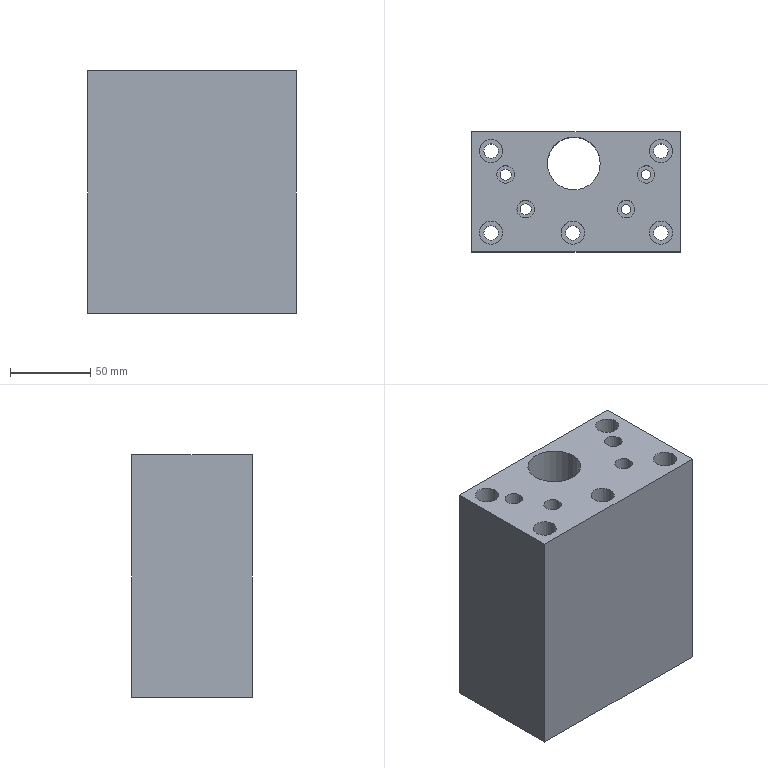Part | NX | features solid 2 | 1 solid | 38 faces | box 130 x 75 x 151.131 mm | volume 1059783 mm3 | cylinder 21 | plane 17 | commonest cylinder face diameters 9.007 x5 14.508 x5 11 x4 6.007 x2 7 x2 41 x2
STEP:
#1=CARTESIAN_POINT('',(1578.267,-85.438,159.999));
#2=VERTEX_POINT('',#1);
#3=CARTESIAN_POINT('',(1581.27,-85.438,159.999));
#4=DIRECTION('',(0.,0.,1.));
#5=DIRECTION('',(-1.,0.,0.));
#6=AXIS2_PLACEMENT_3D('',#3,#4,#5);
#7=CIRCLE('',#6,3.003);
#8=EDGE_CURVE('',#2,#2,#7,.T.);
#9=ORIENTED_EDGE('',*,*,#8,.T.);
#10=EDGE_LOOP('',(#9));
#11=FACE_BOUND('',#10,.T.);
#12=CARTESIAN_POINT('',(1608.02,-74.612,159.999));
#13=VERTEX_POINT('',#12);
#14=CARTESIAN_POINT('',(1587.52,-74.612,159.999));
#15=DIRECTION('',(0.,0.,-1.));
#16=DIRECTION('',(1.,0.,0.));
#17=AXIS2_PLACEMENT_3D('',#14,#15,#16);
#18=CIRCLE('',#17,20.5);
#19=EDGE_CURVE('',#13,#13,#18,.T.);
#20=ORIENTED_EDGE('',*,*,#19,.T.);
#21=EDGE_LOOP('',(#20));
#22=FACE_BOUND('',#21,.T.);
#23=CARTESIAN_POINT('',(1590.767,-63.787,159.999));
#24=VERTEX_POINT('',#23);
#25=CARTESIAN_POINT('',(1593.77,-63.787,159.999));
#26=DIRECTION('',(0.,0.,1.));
#27=DIRECTION('',(-1.,0.,0.));
#28=AXIS2_PLACEMENT_3D('',#25,#26,#27);
#29=CIRCLE('',#28,3.003);
#30=EDGE_CURVE('',#24,#24,#29,.T.);
#31=ORIENTED_EDGE('',*,*,#30,.T.);
#32=EDGE_LOOP('',(#31));
#33=FACE_BOUND('',#32,.T.);
#34=CARTESIAN_POINT('',(1587.52,-74.612,159.999));
#35=DIRECTION('',(0.,0.,-1.));
#36=DIRECTION('',(1.,0.,0.));
#37=AXIS2_PLACEMENT_3D('',#34,#35,#36);
#38=PLANE('',#37);
#39=ADVANCED_FACE('',(#11,#22,#33),#38,.T.);
#40=CARTESIAN_POINT('',(1515.139,-85.438,159.999));
#41=VERTEX_POINT('',#40);
#42=CARTESIAN_POINT('',(1518.639,-85.438,159.999));
#43=DIRECTION('',(0.,0.,-1.));
#44=DIRECTION('',(-1.,0.,0.));
#45=AXIS2_PLACEMENT_3D('',#42,#43,#44);
#46=CIRCLE('',#45,3.5);
#47=EDGE_CURVE('',#41,#41,#46,.F.);
#48=ORIENTED_EDGE('',*,*,#47,.T.);
#49=EDGE_LOOP('',(#48));
#50=FACE_BOUND('',#49,.T.);
#51=CARTESIAN_POINT('',(1532.889,-74.612,159.999));
#52=VERTEX_POINT('',#51);
#53=CARTESIAN_POINT('',(1512.389,-74.612,159.999));
#54=DIRECTION('',(0.,0.,-1.));
#55=DIRECTION('',(1.,0.,0.));
#56=AXIS2_PLACEMENT_3D('',#53,#54,#55);
#57=CIRCLE('',#56,20.5);
#58=EDGE_CURVE('',#52,#52,#57,.T.);
#59=ORIENTED_EDGE('',*,*,#58,.T.);
#60=EDGE_LOOP('',(#59));
#61=FACE_BOUND('',#60,.T.);
#62=CARTESIAN_POINT('',(1502.639,-63.787,159.999));
#63=VERTEX_POINT('',#62);
#64=CARTESIAN_POINT('',(1506.139,-63.787,159.999));
#65=DIRECTION('',(0.,0.,-1.));
#66=DIRECTION('',(-1.,0.,0.));
#67=AXIS2_PLACEMENT_3D('',#64,#65,#66);
#68=CIRCLE('',#67,3.5);
#69=EDGE_CURVE('',#63,#63,#68,.F.);
#70=ORIENTED_EDGE('',*,*,#69,.T.);
#71=EDGE_LOOP('',(#70));
#72=FACE_BOUND('',#71,.T.);
#73=CARTESIAN_POINT('',(1587.52,-74.612,159.999));
#74=DIRECTION('',(0.,0.,-1.));
#75=DIRECTION('',(1.,0.,0.));
#76=AXIS2_PLACEMENT_3D('',#73,#74,#75);
#77=PLANE('',#76);
#78=ADVANCED_FACE('',(#50,#61,#72),#77,.T.);
#79=CARTESIAN_POINT('',(1615.02,-37.112,94.999));
#80=VERTEX_POINT('',#79);
#81=CARTESIAN_POINT('',(1615.02,-37.112,246.13));
#82=VERTEX_POINT('',#81);
#83=CARTESIAN_POINT('',(1615.02,-37.112,184.999));
#84=DIRECTION('',(0.,0.,-1.));
#85=VECTOR('',#84,1000.);
#86=LINE('',#83,#85);
#87=EDGE_CURVE('',#80,#82,#86,.F.);
#88=ORIENTED_EDGE('',*,*,#87,.F.);
#89=CARTESIAN_POINT('',(1485.02,-37.112,94.999));
#90=VERTEX_POINT('',#89);
#91=CARTESIAN_POINT('',(1587.52,-37.112,94.999));
#92=DIRECTION('',(-1.,0.,0.));
#93=VECTOR('',#92,1000.);
#94=LINE('',#91,#93);
#95=EDGE_CURVE('',#80,#90,#94,.T.);
#96=ORIENTED_EDGE('',*,*,#95,.T.);
#97=CARTESIAN_POINT('',(1485.02,-37.112,246.13));
#98=VERTEX_POINT('',#97);
#99=CARTESIAN_POINT('',(1485.02,-37.112,184.999));
#100=DIRECTION('',(0.,0.,-1.));
#101=VECTOR('',#100,1000.);
#102=LINE('',#99,#101);
#103=EDGE_CURVE('',#90,#98,#102,.F.);
#104=ORIENTED_EDGE('',*,*,#103,.T.);
#105=CARTESIAN_POINT('',(1587.52,-37.112,246.13));
#106=DIRECTION('',(-1.,0.,0.));
#107=VECTOR('',#106,1000.);
#108=LINE('',#105,#107);
#109=EDGE_CURVE('',#98,#82,#108,.F.);
#110=ORIENTED_EDGE('',*,*,#109,.T.);
#111=EDGE_LOOP('',(#88,#96,#104,#110));
#112=FACE_BOUND('',#111,.T.);
#113=CARTESIAN_POINT('',(1587.52,-37.112,184.999));
#114=DIRECTION('',(0.,1.,0.));
#115=DIRECTION('',(0.,0.,1.));
#116=AXIS2_PLACEMENT_3D('',#113,#114,#115);
#117=PLANE('',#116);
#118=ADVANCED_FACE('',(#112),#117,.T.);
#119=CARTESIAN_POINT('',(1615.02,-112.112,94.999));
#120=VERTEX_POINT('',#119);
#121=CARTESIAN_POINT('',(1615.02,-112.112,246.13));
#122=VERTEX_POINT('',#121);
#123=CARTESIAN_POINT('',(1615.02,-112.112,184.999));
#124=DIRECTION('',(0.,0.,-1.));
#125=VECTOR('',#124,1000.);
#126=LINE('',#123,#125);
#127=EDGE_CURVE('',#120,#122,#126,.F.);
#128=ORIENTED_EDGE('',*,*,#127,.F.);
#129=CARTESIAN_POINT('',(1615.02,-74.612,94.999));
#130=DIRECTION('',(0.,1.,0.));
#131=VECTOR('',#130,1000.);
#132=LINE('',#129,#131);
#133=EDGE_CURVE('',#120,#80,#132,.T.);
#134=ORIENTED_EDGE('',*,*,#133,.T.);
#135=ORIENTED_EDGE('',*,*,#87,.T.);
#136=CARTESIAN_POINT('',(1615.02,-74.612,246.13));
#137=DIRECTION('',(0.,1.,0.));
#138=VECTOR('',#137,1000.);
#139=LINE('',#136,#138);
#140=EDGE_CURVE('',#82,#122,#139,.F.);
#141=ORIENTED_EDGE('',*,*,#140,.T.);
#142=EDGE_LOOP('',(#128,#134,#135,#141));
#143=FACE_BOUND('',#142,.T.);
#144=CARTESIAN_POINT('',(1615.02,-74.612,184.999));
#145=DIRECTION('',(1.,0.,0.));
#146=DIRECTION('',(0.,0.,-1.));
#147=AXIS2_PLACEMENT_3D('',#144,#145,#146);
#148=PLANE('',#147);
#149=ADVANCED_FACE('',(#143),#148,.T.);
#150=CARTESIAN_POINT('',(1485.02,-112.112,94.999));
#151=VERTEX_POINT('',#150);
#152=CARTESIAN_POINT('',(1485.02,-112.112,246.13));
#153=VERTEX_POINT('',#152);
#154=CARTESIAN_POINT('',(1485.02,-112.112,184.999));
#155=DIRECTION('',(0.,0.,-1.));
#156=VECTOR('',#155,1000.);
#157=LINE('',#154,#156);
#158=EDGE_CURVE('',#151,#153,#157,.F.);
#159=ORIENTED_EDGE('',*,*,#158,.F.);
#160=CARTESIAN_POINT('',(1587.52,-112.112,94.999));
#161=DIRECTION('',(1.,0.,0.));
#162=VECTOR('',#161,1000.);
#163=LINE('',#160,#162);
#164=EDGE_CURVE('',#151,#120,#163,.T.);
#165=ORIENTED_EDGE('',*,*,#164,.T.);
#166=ORIENTED_EDGE('',*,*,#127,.T.);
#167=CARTESIAN_POINT('',(1587.52,-112.112,246.13));
#168=DIRECTION('',(1.,0.,0.));
#169=VECTOR('',#168,1000.);
#170=LINE('',#167,#169);
#171=EDGE_CURVE('',#122,#153,#170,.F.);
#172=ORIENTED_EDGE('',*,*,#171,.T.);
#173=EDGE_LOOP('',(#159,#165,#166,#172));
#174=FACE_BOUND('',#173,.T.);
#175=CARTESIAN_POINT('',(1587.52,-112.112,184.999));
#176=DIRECTION('',(0.,-1.,0.));
#177=DIRECTION('',(0.,0.,-1.));
#178=AXIS2_PLACEMENT_3D('',#175,#176,#177);
#179=PLANE('',#178);
#180=ADVANCED_FACE('',(#174),#179,.T.);
#181=ORIENTED_EDGE('',*,*,#103,.F.);
#182=CARTESIAN_POINT('',(1485.02,-74.612,94.999));
#183=DIRECTION('',(0.,-1.,0.));
#184=VECTOR('',#183,1000.);
#185=LINE('',#182,#184);
#186=EDGE_CURVE('',#90,#151,#185,.T.);
#187=ORIENTED_EDGE('',*,*,#186,.T.);
#188=ORIENTED_EDGE('',*,*,#158,.T.);
#189=CARTESIAN_POINT('',(1485.02,-74.612,246.13));
#190=DIRECTION('',(0.,-1.,0.));
#191=VECTOR('',#190,1000.);
#192=LINE('',#189,#191);
#193=EDGE_CURVE('',#153,#98,#192,.F.);
#194=ORIENTED_EDGE('',*,*,#193,.T.);
#195=EDGE_LOOP('',(#181,#187,#188,#194));
#196=FACE_BOUND('',#195,.T.);
#197=CARTESIAN_POINT('',(1485.02,-74.612,184.999));
#198=DIRECTION('',(-1.,0.,0.));
#199=DIRECTION('',(0.,0.,1.));
#200=AXIS2_PLACEMENT_3D('',#197,#198,#199);
#201=PLANE('',#200);
#202=ADVANCED_FACE('',(#196),#201,.T.);
#203=CARTESIAN_POINT('',(1598.517,-49.112,173.999));
#204=VERTEX_POINT('',#203);
#205=CARTESIAN_POINT('',(1603.02,-49.112,173.999));
#206=DIRECTION('',(0.,0.,1.));
#207=DIRECTION('',(-1.,0.,0.));
#208=AXIS2_PLACEMENT_3D('',#205,#206,#207);
#209=CIRCLE('',#208,4.503);
#210=EDGE_CURVE('',#204,#204,#209,.F.);
#211=ORIENTED_EDGE('',*,*,#210,.F.);
#212=EDGE_LOOP('',(#211));
#213=FACE_BOUND('',#212,.T.);
#214=CARTESIAN_POINT('',(1607.524,-49.112,94.999));
#215=VERTEX_POINT('',#214);
#216=CARTESIAN_POINT('',(1603.02,-49.112,94.999));
#217=DIRECTION('',(0.,0.,-1.));
#218=DIRECTION('',(1.,0.,0.));
#219=AXIS2_PLACEMENT_3D('',#216,#217,#218);
#220=CIRCLE('',#219,4.503);
#221=EDGE_CURVE('',#215,#215,#220,.T.);
#222=ORIENTED_EDGE('',*,*,#221,.T.);
#223=EDGE_LOOP('',(#222));
#224=FACE_BOUND('',#223,.T.);
#225=CARTESIAN_POINT('',(1603.02,-49.112,187.999));
#226=DIRECTION('',(0.,0.,-1.));
#227=DIRECTION('',(-1.,0.,0.));
#228=AXIS2_PLACEMENT_3D('',#225,#226,#227);
#229=CYLINDRICAL_SURFACE('',#228,4.503);
#230=ADVANCED_FACE('',(#213,#224),#229,.F.);
#231=CARTESIAN_POINT('',(1492.517,-100.112,173.999));
#232=VERTEX_POINT('',#231);
#233=CARTESIAN_POINT('',(1497.02,-100.112,173.999));
#234=DIRECTION('',(0.,0.,1.));
#235=DIRECTION('',(-1.,0.,0.));
#236=AXIS2_PLACEMENT_3D('',#233,#234,#235);
#237=CIRCLE('',#236,4.503);
#238=EDGE_CURVE('',#232,#232,#237,.F.);
#239=ORIENTED_EDGE('',*,*,#238,.F.);
#240=EDGE_LOOP('',(#239));
#241=FACE_BOUND('',#240,.T.);
#242=CARTESIAN_POINT('',(1501.524,-100.112,94.999));
#243=VERTEX_POINT('',#242);
#244=CARTESIAN_POINT('',(1497.02,-100.112,94.999));
#245=DIRECTION('',(0.,0.,-1.));
#246=DIRECTION('',(1.,0.,0.));
#247=AXIS2_PLACEMENT_3D('',#244,#245,#246);
#248=CIRCLE('',#247,4.503);
#249=EDGE_CURVE('',#243,#243,#248,.T.);
#250=ORIENTED_EDGE('',*,*,#249,.T.);
#251=EDGE_LOOP('',(#250));
#252=FACE_BOUND('',#251,.T.);
#253=CARTESIAN_POINT('',(1497.02,-100.112,187.999));
#254=DIRECTION('',(0.,0.,-1.));
#255=DIRECTION('',(-1.,0.,0.));
#256=AXIS2_PLACEMENT_3D('',#253,#254,#255);
#257=CYLINDRICAL_SURFACE('',#256,4.503);
#258=ADVANCED_FACE('',(#241,#252),#257,.F.);
#259=CARTESIAN_POINT('',(1492.517,-49.112,173.999));
#260=VERTEX_POINT('',#259);
#261=CARTESIAN_POINT('',(1497.02,-49.112,173.999));
#262=DIRECTION('',(0.,0.,1.));
#263=DIRECTION('',(-1.,0.,0.));
#264=AXIS2_PLACEMENT_3D('',#261,#262,#263);
#265=CIRCLE('',#264,4.503);
#266=EDGE_CURVE('',#260,#260,#265,.F.);
#267=ORIENTED_EDGE('',*,*,#266,.F.);
#268=EDGE_LOOP('',(#267));
#269=FACE_BOUND('',#268,.T.);
#270=CARTESIAN_POINT('',(1501.524,-49.112,94.999));
#271=VERTEX_POINT('',#270);
#272=CARTESIAN_POINT('',(1497.02,-49.112,94.999));
#273=DIRECTION('',(0.,0.,-1.));
#274=DIRECTION('',(1.,0.,0.));
#275=AXIS2_PLACEMENT_3D('',#272,#273,#274);
#276=CIRCLE('',#275,4.503);
#277=EDGE_CURVE('',#271,#271,#276,.T.);
#278=ORIENTED_EDGE('',*,*,#277,.T.);
#279=EDGE_LOOP('',(#278));
#280=FACE_BOUND('',#279,.T.);
#281=CARTESIAN_POINT('',(1497.02,-49.112,187.999));
#282=DIRECTION('',(0.,0.,-1.));
#283=DIRECTION('',(-1.,0.,0.));
#284=AXIS2_PLACEMENT_3D('',#281,#282,#283);
#285=CYLINDRICAL_SURFACE('',#284,4.503);
#286=ADVANCED_FACE('',(#269,#280),#285,.F.);
#287=CARTESIAN_POINT('',(1598.517,-100.112,173.999));
#288=VERTEX_POINT('',#287);
#289=CARTESIAN_POINT('',(1603.02,-100.112,173.999));
#290=DIRECTION('',(0.,0.,1.));
#291=DIRECTION('',(-1.,0.,0.));
#292=AXIS2_PLACEMENT_3D('',#289,#290,#291);
#293=CIRCLE('',#292,4.503);
#294=EDGE_CURVE('',#288,#288,#293,.F.);
#295=ORIENTED_EDGE('',*,*,#294,.F.);
#296=EDGE_LOOP('',(#295));
#297=FACE_BOUND('',#296,.T.);
#298=CARTESIAN_POINT('',(1607.524,-100.112,94.999));
#299=VERTEX_POINT('',#298);
#300=CARTESIAN_POINT('',(1603.02,-100.112,94.999));
#301=DIRECTION('',(0.,0.,-1.));
#302=DIRECTION('',(1.,0.,0.));
#303=AXIS2_PLACEMENT_3D('',#300,#301,#302);
#304=CIRCLE('',#303,4.503);
#305=EDGE_CURVE('',#299,#299,#304,.T.);
#306=ORIENTED_EDGE('',*,*,#305,.T.);
#307=EDGE_LOOP('',(#306));
#308=FACE_BOUND('',#307,.T.);
#309=CARTESIAN_POINT('',(1603.02,-100.112,187.999));
#310=DIRECTION('',(0.,0.,-1.));
#311=DIRECTION('',(-1.,0.,0.));
#312=AXIS2_PLACEMENT_3D('',#309,#310,#311);
#313=CYLINDRICAL_SURFACE('',#312,4.503);
#314=ADVANCED_FACE('',(#297,#308),#313,.F.);
#315=CARTESIAN_POINT('',(1543.517,-100.112,173.999));
#316=VERTEX_POINT('',#315);
#317=CARTESIAN_POINT('',(1548.02,-100.112,173.999));
#318=DIRECTION('',(0.,0.,1.));
#319=DIRECTION('',(-1.,0.,0.));
#320=AXIS2_PLACEMENT_3D('',#317,#318,#319);
#321=CIRCLE('',#320,4.503);
#322=EDGE_CURVE('',#316,#316,#321,.F.);
#323=ORIENTED_EDGE('',*,*,#322,.F.);
#324=EDGE_LOOP('',(#323));
#325=FACE_BOUND('',#324,.T.);
#326=CARTESIAN_POINT('',(1552.524,-100.112,94.999));
#327=VERTEX_POINT('',#326);
#328=CARTESIAN_POINT('',(1548.02,-100.112,94.999));
#329=DIRECTION('',(0.,0.,-1.));
#330=DIRECTION('',(1.,0.,0.));
#331=AXIS2_PLACEMENT_3D('',#328,#329,#330);
#332=CIRCLE('',#331,4.503);
#333=EDGE_CURVE('',#327,#327,#332,.F.);
#334=ORIENTED_EDGE('',*,*,#333,.F.);
#335=EDGE_LOOP('',(#334));
#336=FACE_BOUND('',#335,.T.);
#337=CARTESIAN_POINT('',(1548.02,-100.112,187.999));
#338=DIRECTION('',(0.,0.,-1.));
#339=DIRECTION('',(-1.,0.,0.));
#340=AXIS2_PLACEMENT_3D('',#337,#338,#339);
#341=CYLINDRICAL_SURFACE('',#340,4.503);
#342=ADVANCED_FACE('',(#325,#336),#341,.F.);
#343=CARTESIAN_POINT('',(1532.146,-56.913,246.13));
#344=VERTEX_POINT('',#343);
#345=CARTESIAN_POINT('',(1548.646,-56.913,246.13));
#346=DIRECTION('',(0.,0.,-1.));
#347=DIRECTION('',(-1.,0.,0.));
#348=AXIS2_PLACEMENT_3D('',#345,#346,#347);
#349=CIRCLE('',#348,16.5);
#350=EDGE_CURVE('',#344,#344,#349,.T.);
#351=ORIENTED_EDGE('',*,*,#350,.F.);
#352=EDGE_LOOP('',(#351));
#353=FACE_BOUND('',#352,.T.);
#354=CARTESIAN_POINT('',(1565.146,-56.913,94.999));
#355=VERTEX_POINT('',#354);
#356=CARTESIAN_POINT('',(1548.646,-56.913,94.999));
#357=DIRECTION('',(0.,0.,-1.));
#358=DIRECTION('',(1.,0.,0.));
#359=AXIS2_PLACEMENT_3D('',#356,#357,#358);
#360=CIRCLE('',#359,16.5);
#361=EDGE_CURVE('',#355,#355,#360,.F.);
#362=ORIENTED_EDGE('',*,*,#361,.F.);
#363=EDGE_LOOP('',(#362));
#364=FACE_BOUND('',#363,.T.);
#365=CARTESIAN_POINT('',(1548.646,-56.913,-109.999));
#366=DIRECTION('',(0.,0.,1.));
#367=DIRECTION('',(-1.,0.,0.));
#368=AXIS2_PLACEMENT_3D('',#365,#366,#367);
#369=CYLINDRICAL_SURFACE('',#368,16.5);
#370=ADVANCED_FACE('',(#353,#364),#369,.F.);
#371=CARTESIAN_POINT('',(1588.27,-63.787,246.13));
#372=VERTEX_POINT('',#371);
#373=CARTESIAN_POINT('',(1593.77,-63.787,246.13));
#374=DIRECTION('',(0.,0.,-1.));
#375=DIRECTION('',(-1.,0.,0.));
#376=AXIS2_PLACEMENT_3D('',#373,#374,#375);
#377=CIRCLE('',#376,5.5);
#378=EDGE_CURVE('',#372,#372,#377,.F.);
#379=ORIENTED_EDGE('',*,*,#378,.F.);
#380=EDGE_LOOP('',(#379));
#381=FACE_BOUND('',#380,.T.);
#382=CARTESIAN_POINT('',(1575.77,-85.438,246.13));
#383=VERTEX_POINT('',#382);
#384=CARTESIAN_POINT('',(1581.27,-85.438,246.13));
#385=DIRECTION('',(0.,0.,-1.));
#386=DIRECTION('',(-1.,0.,0.));
#387=AXIS2_PLACEMENT_3D('',#384,#385,#386);
#388=CIRCLE('',#387,5.5);
#389=EDGE_CURVE('',#383,#383,#388,.F.);
#390=ORIENTED_EDGE('',*,*,#389,.F.);
#391=EDGE_LOOP('',(#390));
#392=FACE_BOUND('',#391,.T.);
#393=CARTESIAN_POINT('',(1500.639,-63.787,246.13));
#394=VERTEX_POINT('',#393);
#395=CARTESIAN_POINT('',(1506.139,-63.787,246.13));
#396=DIRECTION('',(0.,0.,-1.));
#397=DIRECTION('',(-1.,0.,0.));
#398=AXIS2_PLACEMENT_3D('',#395,#396,#397);
#399=CIRCLE('',#398,5.5);
#400=EDGE_CURVE('',#394,#394,#399,.F.);
#401=ORIENTED_EDGE('',*,*,#400,.F.);
#402=EDGE_LOOP('',(#401));
#403=FACE_BOUND('',#402,.T.);
#404=CARTESIAN_POINT('',(1513.139,-85.438,246.13));
#405=VERTEX_POINT('',#404);
#406=CARTESIAN_POINT('',(1518.639,-85.438,246.13));
#407=DIRECTION('',(0.,0.,-1.));
#408=DIRECTION('',(-1.,0.,0.));
#409=AXIS2_PLACEMENT_3D('',#406,#407,#408);
#410=CIRCLE('',#409,5.5);
#411=EDGE_CURVE('',#405,#405,#410,.F.);
#412=ORIENTED_EDGE('',*,*,#411,.F.);
#413=EDGE_LOOP('',(#412));
#414=FACE_BOUND('',#413,.T.);
#415=CARTESIAN_POINT('',(1595.766,-100.112,246.13));
#416=VERTEX_POINT('',#415);
#417=CARTESIAN_POINT('',(1603.02,-100.112,246.13));
#418=DIRECTION('',(0.,0.,-1.));
#419=DIRECTION('',(-1.,0.,0.));
#420=AXIS2_PLACEMENT_3D('',#417,#418,#419);
#421=CIRCLE('',#420,7.254);
#422=EDGE_CURVE('',#416,#416,#421,.T.);
#423=ORIENTED_EDGE('',*,*,#422,.T.);
#424=EDGE_LOOP('',(#423));
#425=FACE_BOUND('',#424,.T.);
#426=CARTESIAN_POINT('',(1489.766,-100.112,246.13));
#427=VERTEX_POINT('',#426);
#428=CARTESIAN_POINT('',(1497.02,-100.112,246.13));
#429=DIRECTION('',(0.,0.,-1.));
#430=DIRECTION('',(-1.,0.,0.));
#431=AXIS2_PLACEMENT_3D('',#428,#429,#430);
#432=CIRCLE('',#431,7.254);
#433=EDGE_CURVE('',#427,#427,#432,.T.);
#434=ORIENTED_EDGE('',*,*,#433,.T.);
#435=EDGE_LOOP('',(#434));
#436=FACE_BOUND('',#435,.T.);
#437=ORIENTED_EDGE('',*,*,#193,.F.);
#438=ORIENTED_EDGE('',*,*,#171,.F.);
#439=ORIENTED_EDGE('',*,*,#140,.F.);
#440=ORIENTED_EDGE('',*,*,#109,.F.);
#441=EDGE_LOOP('',(#437,#438,#439,#440));
#442=FACE_BOUND('',#441,.T.);
#443=CARTESIAN_POINT('',(1595.766,-49.112,246.13));
#444=VERTEX_POINT('',#443);
#445=CARTESIAN_POINT('',(1603.02,-49.112,246.13));
#446=DIRECTION('',(0.,0.,-1.));
#447=DIRECTION('',(-1.,0.,0.));
#448=AXIS2_PLACEMENT_3D('',#445,#446,#447);
#449=CIRCLE('',#448,7.254);
#450=EDGE_CURVE('',#444,#444,#449,.T.);
#451=ORIENTED_EDGE('',*,*,#450,.T.);
#452=EDGE_LOOP('',(#451));
#453=FACE_BOUND('',#452,.T.);
#454=CARTESIAN_POINT('',(1489.766,-49.112,246.13));
#455=VERTEX_POINT('',#454);
#456=CARTESIAN_POINT('',(1497.02,-49.112,246.13));
#457=DIRECTION('',(0.,0.,-1.));
#458=DIRECTION('',(-1.,0.,0.));
#459=AXIS2_PLACEMENT_3D('',#456,#457,#458);
#460=CIRCLE('',#459,7.254);
#461=EDGE_CURVE('',#455,#455,#460,.T.);
#462=ORIENTED_EDGE('',*,*,#461,.T.);
#463=EDGE_LOOP('',(#462));
#464=FACE_BOUND('',#463,.T.);
#465=CARTESIAN_POINT('',(1540.766,-100.112,246.13));
#466=VERTEX_POINT('',#465);
#467=CARTESIAN_POINT('',(1548.02,-100.112,246.13));
#468=DIRECTION('',(0.,0.,-1.));
#469=DIRECTION('',(-1.,0.,0.));
#470=AXIS2_PLACEMENT_3D('',#467,#468,#469);
#471=CIRCLE('',#470,7.254);
#472=EDGE_CURVE('',#466,#466,#471,.T.);
#473=ORIENTED_EDGE('',*,*,#472,.T.);
#474=EDGE_LOOP('',(#473));
#475=FACE_BOUND('',#474,.T.);
#476=ORIENTED_EDGE('',*,*,#350,.T.);
#477=EDGE_LOOP('',(#476));
#478=FACE_BOUND('',#477,.T.);
#479=CARTESIAN_POINT('',(3499.955,4.191,246.13));
#480=DIRECTION('',(0.,0.,-1.));
#481=DIRECTION('',(1.,0.,0.));
#482=AXIS2_PLACEMENT_3D('',#479,#480,#481);
#483=PLANE('',#482);
#484=ADVANCED_FACE('',(#381,#392,#403,#414,#425,#436,#442,#453,#464,#475,#478),#483,.F.);
#485=ORIENTED_EDGE('',*,*,#210,.T.);
#486=EDGE_LOOP('',(#485));
#487=FACE_BOUND('',#486,.T.);
#488=CARTESIAN_POINT('',(1595.766,-49.112,173.999));
#489=VERTEX_POINT('',#488);
#490=CARTESIAN_POINT('',(1603.02,-49.112,173.999));
#491=DIRECTION('',(0.,0.,-1.));
#492=DIRECTION('',(-1.,0.,0.));
#493=AXIS2_PLACEMENT_3D('',#490,#491,#492);
#494=CIRCLE('',#493,7.254);
#495=EDGE_CURVE('',#489,#489,#494,.T.);
#496=ORIENTED_EDGE('',*,*,#495,.F.);
#497=EDGE_LOOP('',(#496));
#498=FACE_BOUND('',#497,.T.);
#499=CARTESIAN_POINT('',(1603.02,-49.112,173.999));
#500=DIRECTION('',(0.,0.,-1.));
#501=DIRECTION('',(-1.,0.,0.));
#502=AXIS2_PLACEMENT_3D('',#499,#500,#501);
#503=PLANE('',#502);
#504=ADVANCED_FACE('',(#487,#498),#503,.F.);
#505=ORIENTED_EDGE('',*,*,#495,.T.);
#506=EDGE_LOOP('',(#505));
#507=FACE_BOUND('',#506,.T.);
#508=ORIENTED_EDGE('',*,*,#450,.F.);
#509=EDGE_LOOP('',(#508));
#510=FACE_BOUND('',#509,.T.);
#511=CARTESIAN_POINT('',(1603.02,-49.112,184.999));
#512=DIRECTION('',(0.,0.,-1.));
#513=DIRECTION('',(-1.,0.,0.));
#514=AXIS2_PLACEMENT_3D('',#511,#512,#513);
#515=CYLINDRICAL_SURFACE('',#514,7.254);
#516=ADVANCED_FACE('',(#507,#510),#515,.F.);
#517=ORIENTED_EDGE('',*,*,#238,.T.);
#518=EDGE_LOOP('',(#517));
#519=FACE_BOUND('',#518,.T.);
#520=CARTESIAN_POINT('',(1489.766,-100.112,173.999));
#521=VERTEX_POINT('',#520);
#522=CARTESIAN_POINT('',(1497.02,-100.112,173.999));
#523=DIRECTION('',(0.,0.,-1.));
#524=DIRECTION('',(-1.,0.,0.));
#525=AXIS2_PLACEMENT_3D('',#522,#523,#524);
#526=CIRCLE('',#525,7.254);
#527=EDGE_CURVE('',#521,#521,#526,.T.);
#528=ORIENTED_EDGE('',*,*,#527,.F.);
#529=EDGE_LOOP('',(#528));
#530=FACE_BOUND('',#529,.T.);
#531=CARTESIAN_POINT('',(1497.02,-100.112,173.999));
#532=DIRECTION('',(0.,0.,-1.));
#533=DIRECTION('',(-1.,0.,0.));
#534=AXIS2_PLACEMENT_3D('',#531,#532,#533);
#535=PLANE('',#534);
#536=ADVANCED_FACE('',(#519,#530),#535,.F.);
#537=ORIENTED_EDGE('',*,*,#527,.T.);
#538=EDGE_LOOP('',(#537));
#539=FACE_BOUND('',#538,.T.);
#540=ORIENTED_EDGE('',*,*,#433,.F.);
#541=EDGE_LOOP('',(#540));
#542=FACE_BOUND('',#541,.T.);
#543=CARTESIAN_POINT('',(1497.02,-100.112,184.999));
#544=DIRECTION('',(0.,0.,-1.));
#545=DIRECTION('',(-1.,0.,0.));
#546=AXIS2_PLACEMENT_3D('',#543,#544,#545);
#547=CYLINDRICAL_SURFACE('',#546,7.254);
#548=ADVANCED_FACE('',(#539,#542),#547,.F.);
#549=ORIENTED_EDGE('',*,*,#266,.T.);
#550=EDGE_LOOP('',(#549));
#551=FACE_BOUND('',#550,.T.);
#552=CARTESIAN_POINT('',(1489.766,-49.112,173.999));
#553=VERTEX_POINT('',#552);
#554=CARTESIAN_POINT('',(1497.02,-49.112,173.999));
#555=DIRECTION('',(0.,0.,-1.));
#556=DIRECTION('',(-1.,0.,0.));
#557=AXIS2_PLACEMENT_3D('',#554,#555,#556);
#558=CIRCLE('',#557,7.254);
#559=EDGE_CURVE('',#553,#553,#558,.T.);
#560=ORIENTED_EDGE('',*,*,#559,.F.);
#561=EDGE_LOOP('',(#560));
#562=FACE_BOUND('',#561,.T.);
#563=CARTESIAN_POINT('',(1497.02,-49.112,173.999));
#564=DIRECTION('',(0.,0.,-1.));
#565=DIRECTION('',(-1.,0.,0.));
#566=AXIS2_PLACEMENT_3D('',#563,#564,#565);
#567=PLANE('',#566);
#568=ADVANCED_FACE('',(#551,#562),#567,.F.);
#569=ORIENTED_EDGE('',*,*,#559,.T.);
#570=EDGE_LOOP('',(#569));
#571=FACE_BOUND('',#570,.T.);
#572=ORIENTED_EDGE('',*,*,#461,.F.);
#573=EDGE_LOOP('',(#572));
#574=FACE_BOUND('',#573,.T.);
#575=CARTESIAN_POINT('',(1497.02,-49.112,184.999));
#576=DIRECTION('',(0.,0.,-1.));
#577=DIRECTION('',(-1.,0.,0.));
#578=AXIS2_PLACEMENT_3D('',#575,#576,#577);
#579=CYLINDRICAL_SURFACE('',#578,7.254);
#580=ADVANCED_FACE('',(#571,#574),#579,.F.);
#581=ORIENTED_EDGE('',*,*,#294,.T.);
#582=EDGE_LOOP('',(#581));
#583=FACE_BOUND('',#582,.T.);
#584=CARTESIAN_POINT('',(1595.766,-100.112,173.999));
#585=VERTEX_POINT('',#584);
#586=CARTESIAN_POINT('',(1603.02,-100.112,173.999));
#587=DIRECTION('',(0.,0.,-1.));
#588=DIRECTION('',(-1.,0.,0.));
#589=AXIS2_PLACEMENT_3D('',#586,#587,#588);
#590=CIRCLE('',#589,7.254);
#591=EDGE_CURVE('',#585,#585,#590,.T.);
#592=ORIENTED_EDGE('',*,*,#591,.F.);
#593=EDGE_LOOP('',(#592));
#594=FACE_BOUND('',#593,.T.);
#595=CARTESIAN_POINT('',(1603.02,-100.112,173.999));
#596=DIRECTION('',(0.,0.,-1.));
#597=DIRECTION('',(-1.,0.,0.));
#598=AXIS2_PLACEMENT_3D('',#595,#596,#597);
#599=PLANE('',#598);
#600=ADVANCED_FACE('',(#583,#594),#599,.F.);
#601=ORIENTED_EDGE('',*,*,#591,.T.);
#602=EDGE_LOOP('',(#601));
#603=FACE_BOUND('',#602,.T.);
#604=ORIENTED_EDGE('',*,*,#422,.F.);
#605=EDGE_LOOP('',(#604));
#606=FACE_BOUND('',#605,.T.);
#607=CARTESIAN_POINT('',(1603.02,-100.112,184.999));
#608=DIRECTION('',(0.,0.,-1.));
#609=DIRECTION('',(-1.,0.,0.));
#610=AXIS2_PLACEMENT_3D('',#607,#608,#609);
#611=CYLINDRICAL_SURFACE('',#610,7.254);
#612=ADVANCED_FACE('',(#603,#606),#611,.F.);
#613=ORIENTED_EDGE('',*,*,#322,.T.);
#614=EDGE_LOOP('',(#613));
#615=FACE_BOUND('',#614,.T.);
#616=CARTESIAN_POINT('',(1540.766,-100.112,173.999));
#617=VERTEX_POINT('',#616);
#618=CARTESIAN_POINT('',(1548.02,-100.112,173.999));
#619=DIRECTION('',(0.,0.,-1.));
#620=DIRECTION('',(-1.,0.,0.));
#621=AXIS2_PLACEMENT_3D('',#618,#619,#620);
#622=CIRCLE('',#621,7.254);
#623=EDGE_CURVE('',#617,#617,#622,.T.);
#624=ORIENTED_EDGE('',*,*,#623,.F.);
#625=EDGE_LOOP('',(#624));
#626=FACE_BOUND('',#625,.T.);
#627=CARTESIAN_POINT('',(1548.02,-100.112,173.999));
#628=DIRECTION('',(0.,0.,-1.));
#629=DIRECTION('',(-1.,0.,0.));
#630=AXIS2_PLACEMENT_3D('',#627,#628,#629);
#631=PLANE('',#630);
#632=ADVANCED_FACE('',(#615,#626),#631,.F.);
#633=ORIENTED_EDGE('',*,*,#623,.T.);
#634=EDGE_LOOP('',(#633));
#635=FACE_BOUND('',#634,.T.);
#636=ORIENTED_EDGE('',*,*,#472,.F.);
#637=EDGE_LOOP('',(#636));
#638=FACE_BOUND('',#637,.T.);
#639=CARTESIAN_POINT('',(1548.02,-100.112,184.999));
#640=DIRECTION('',(0.,0.,-1.));
#641=DIRECTION('',(-1.,0.,0.));
#642=AXIS2_PLACEMENT_3D('',#639,#640,#641);
#643=CYLINDRICAL_SURFACE('',#642,7.254);
#644=ADVANCED_FACE('',(#635,#638),#643,.F.);
#645=CARTESIAN_POINT('',(1532.889,-74.612,94.999));
#646=VERTEX_POINT('',#645);
#647=CARTESIAN_POINT('',(1512.389,-74.612,94.999));
#648=DIRECTION('',(0.,0.,-1.));
#649=DIRECTION('',(1.,0.,0.));
#650=AXIS2_PLACEMENT_3D('',#647,#648,#649);
#651=CIRCLE('',#650,20.5);
#652=EDGE_CURVE('',#646,#646,#651,.F.);
#653=ORIENTED_EDGE('',*,*,#652,.F.);
#654=EDGE_LOOP('',(#653));
#655=FACE_BOUND('',#654,.T.);
#656=ORIENTED_EDGE('',*,*,#58,.F.);
#657=EDGE_LOOP('',(#656));
#658=FACE_BOUND('',#657,.T.);
#659=CARTESIAN_POINT('',(1512.389,-74.612,1037.539));
#660=DIRECTION('',(0.,0.,-1.));
#661=DIRECTION('',(-0.5,0.866,0.));
#662=AXIS2_PLACEMENT_3D('',#659,#660,#661);
#663=CYLINDRICAL_SURFACE('',#662,20.5);
#664=ADVANCED_FACE('',(#655,#658),#663,.F.);
#665=ORIENTED_EDGE('',*,*,#652,.T.);
#666=EDGE_LOOP('',(#665));
#667=FACE_BOUND('',#666,.T.);
#668=ORIENTED_EDGE('',*,*,#95,.F.);
#669=ORIENTED_EDGE('',*,*,#133,.F.);
#670=ORIENTED_EDGE('',*,*,#164,.F.);
#671=ORIENTED_EDGE('',*,*,#186,.F.);
#672=EDGE_LOOP('',(#668,#669,#670,#671));
#673=FACE_BOUND('',#672,.T.);
#674=ORIENTED_EDGE('',*,*,#221,.F.);
#675=EDGE_LOOP('',(#674));
#676=FACE_BOUND('',#675,.T.);
#677=ORIENTED_EDGE('',*,*,#249,.F.);
#678=EDGE_LOOP('',(#677));
#679=FACE_BOUND('',#678,.T.);
#680=ORIENTED_EDGE('',*,*,#277,.F.);
#681=EDGE_LOOP('',(#680));
#682=FACE_BOUND('',#681,.T.);
#683=ORIENTED_EDGE('',*,*,#305,.F.);
#684=EDGE_LOOP('',(#683));
#685=FACE_BOUND('',#684,.T.);
#686=ORIENTED_EDGE('',*,*,#333,.T.);
#687=EDGE_LOOP('',(#686));
#688=FACE_BOUND('',#687,.T.);
#689=ORIENTED_EDGE('',*,*,#361,.T.);
#690=EDGE_LOOP('',(#689));
#691=FACE_BOUND('',#690,.T.);
#692=CARTESIAN_POINT('',(1608.02,-74.612,94.999));
#693=VERTEX_POINT('',#692);
#694=CARTESIAN_POINT('',(1587.52,-74.612,94.999));
#695=DIRECTION('',(0.,0.,-1.));
#696=DIRECTION('',(1.,0.,0.));
#697=AXIS2_PLACEMENT_3D('',#694,#695,#696);
#698=CIRCLE('',#697,20.5);
#699=EDGE_CURVE('',#693,#693,#698,.F.);
#700=ORIENTED_EDGE('',*,*,#699,.T.);
#701=EDGE_LOOP('',(#700));
#702=FACE_BOUND('',#701,.T.);
#703=CARTESIAN_POINT('',(1554.955,6.94,94.999));
#704=DIRECTION('',(0.,0.,-1.));
#705=DIRECTION('',(-1.,0.,0.));
#706=AXIS2_PLACEMENT_3D('',#703,#704,#705);
#707=PLANE('',#706);
#708=ADVANCED_FACE('',(#667,#673,#676,#679,#682,#685,#688,#691,#702),#707,.T.);
#709=ORIENTED_EDGE('',*,*,#699,.F.);
#710=EDGE_LOOP('',(#709));
#711=FACE_BOUND('',#710,.T.);
#712=ORIENTED_EDGE('',*,*,#19,.F.);
#713=EDGE_LOOP('',(#712));
#714=FACE_BOUND('',#713,.T.);
#715=CARTESIAN_POINT('',(1587.52,-74.612,1037.539));
#716=DIRECTION('',(0.,0.,-1.));
#717=DIRECTION('',(0.5,0.866,0.));
#718=AXIS2_PLACEMENT_3D('',#715,#716,#717);
#719=CYLINDRICAL_SURFACE('',#718,20.5);
#720=ADVANCED_FACE('',(#711,#714),#719,.F.);
#721=ORIENTED_EDGE('',*,*,#47,.F.);
#722=EDGE_LOOP('',(#721));
#723=FACE_BOUND('',#722,.T.);
#724=CARTESIAN_POINT('',(1515.139,-85.438,178.999));
#725=VERTEX_POINT('',#724);
#726=CARTESIAN_POINT('',(1518.639,-85.438,178.999));
#727=DIRECTION('',(0.,0.,-1.));
#728=DIRECTION('',(-1.,0.,0.));
#729=AXIS2_PLACEMENT_3D('',#726,#727,#728);
#730=CIRCLE('',#729,3.5);
#731=EDGE_CURVE('',#725,#725,#730,.T.);
#732=ORIENTED_EDGE('',*,*,#731,.F.);
#733=EDGE_LOOP('',(#732));
#734=FACE_BOUND('',#733,.T.);
#735=CARTESIAN_POINT('',(1518.639,-85.438,201.999));
#736=DIRECTION('',(0.,0.,-1.));
#737=DIRECTION('',(-1.,0.,0.));
#738=AXIS2_PLACEMENT_3D('',#735,#736,#737);
#739=CYLINDRICAL_SURFACE('',#738,3.5);
#740=ADVANCED_FACE('',(#723,#734),#739,.F.);
#741=ORIENTED_EDGE('',*,*,#731,.T.);
#742=EDGE_LOOP('',(#741));
#743=FACE_BOUND('',#742,.T.);
#744=CARTESIAN_POINT('',(1513.139,-85.438,178.999));
#745=VERTEX_POINT('',#744);
#746=CARTESIAN_POINT('',(1518.639,-85.438,178.999));
#747=DIRECTION('',(0.,0.,-1.));
#748=DIRECTION('',(-1.,0.,0.));
#749=AXIS2_PLACEMENT_3D('',#746,#747,#748);
#750=CIRCLE('',#749,5.5);
#751=EDGE_CURVE('',#745,#745,#750,.T.);
#752=ORIENTED_EDGE('',*,*,#751,.F.);
#753=EDGE_LOOP('',(#752));
#754=FACE_BOUND('',#753,.T.);
#755=CARTESIAN_POINT('',(1518.639,-85.438,178.999));
#756=DIRECTION('',(0.,0.,-1.));
#757=DIRECTION('',(1.,0.,0.));
#758=AXIS2_PLACEMENT_3D('',#755,#756,#757);
#759=PLANE('',#758);
#760=ADVANCED_FACE('',(#743,#754),#759,.F.);
#761=ORIENTED_EDGE('',*,*,#411,.T.);
#762=EDGE_LOOP('',(#761));
#763=FACE_BOUND('',#762,.T.);
#764=ORIENTED_EDGE('',*,*,#751,.T.);
#765=EDGE_LOOP('',(#764));
#766=FACE_BOUND('',#765,.T.);
#767=CARTESIAN_POINT('',(1518.639,-85.438,201.999));
#768=DIRECTION('',(0.,0.,-1.));
#769=DIRECTION('',(-1.,0.,0.));
#770=AXIS2_PLACEMENT_3D('',#767,#768,#769);
#771=CYLINDRICAL_SURFACE('',#770,5.5);
#772=ADVANCED_FACE('',(#763,#766),#771,.F.);
#773=ORIENTED_EDGE('',*,*,#69,.F.);
#774=EDGE_LOOP('',(#773));
#775=FACE_BOUND('',#774,.T.);
#776=CARTESIAN_POINT('',(1502.639,-63.787,178.999));
#777=VERTEX_POINT('',#776);
#778=CARTESIAN_POINT('',(1506.139,-63.787,178.999));
#779=DIRECTION('',(0.,0.,-1.));
#780=DIRECTION('',(-1.,0.,0.));
#781=AXIS2_PLACEMENT_3D('',#778,#779,#780);
#782=CIRCLE('',#781,3.5);
#783=EDGE_CURVE('',#777,#777,#782,.T.);
#784=ORIENTED_EDGE('',*,*,#783,.F.);
#785=EDGE_LOOP('',(#784));
#786=FACE_BOUND('',#785,.T.);
#787=CARTESIAN_POINT('',(1506.139,-63.787,201.999));
#788=DIRECTION('',(0.,0.,-1.));
#789=DIRECTION('',(-1.,0.,0.));
#790=AXIS2_PLACEMENT_3D('',#787,#788,#789);
#791=CYLINDRICAL_SURFACE('',#790,3.5);
#792=ADVANCED_FACE('',(#775,#786),#791,.F.);
#793=ORIENTED_EDGE('',*,*,#783,.T.);
#794=EDGE_LOOP('',(#793));
#795=FACE_BOUND('',#794,.T.);
#796=CARTESIAN_POINT('',(1500.639,-63.787,178.999));
#797=VERTEX_POINT('',#796);
#798=CARTESIAN_POINT('',(1506.139,-63.787,178.999));
#799=DIRECTION('',(0.,0.,-1.));
#800=DIRECTION('',(-1.,0.,0.));
#801=AXIS2_PLACEMENT_3D('',#798,#799,#800);
#802=CIRCLE('',#801,5.5);
#803=EDGE_CURVE('',#797,#797,#802,.T.);
#804=ORIENTED_EDGE('',*,*,#803,.F.);
#805=EDGE_LOOP('',(#804));
#806=FACE_BOUND('',#805,.T.);
#807=CARTESIAN_POINT('',(1506.139,-63.787,178.999));
#808=DIRECTION('',(0.,0.,-1.));
#809=DIRECTION('',(1.,0.,0.));
#810=AXIS2_PLACEMENT_3D('',#807,#808,#809);
#811=PLANE('',#810);
#812=ADVANCED_FACE('',(#795,#806),#811,.F.);
#813=ORIENTED_EDGE('',*,*,#400,.T.);
#814=EDGE_LOOP('',(#813));
#815=FACE_BOUND('',#814,.T.);
#816=ORIENTED_EDGE('',*,*,#803,.T.);
#817=EDGE_LOOP('',(#816));
#818=FACE_BOUND('',#817,.T.);
#819=CARTESIAN_POINT('',(1506.139,-63.787,201.999));
#820=DIRECTION('',(0.,0.,-1.));
#821=DIRECTION('',(-1.,0.,0.));
#822=AXIS2_PLACEMENT_3D('',#819,#820,#821);
#823=CYLINDRICAL_SURFACE('',#822,5.5);
#824=ADVANCED_FACE('',(#815,#818),#823,.F.);
#825=ORIENTED_EDGE('',*,*,#8,.F.);
#826=EDGE_LOOP('',(#825));
#827=FACE_BOUND('',#826,.T.);
#828=CARTESIAN_POINT('',(1584.274,-85.438,178.999));
#829=VERTEX_POINT('',#828);
#830=CARTESIAN_POINT('',(1581.27,-85.438,178.999));
#831=DIRECTION('',(0.,0.,-1.));
#832=DIRECTION('',(1.,0.,0.));
#833=AXIS2_PLACEMENT_3D('',#830,#831,#832);
#834=CIRCLE('',#833,3.003);
#835=EDGE_CURVE('',#829,#829,#834,.T.);
#836=ORIENTED_EDGE('',*,*,#835,.F.);
#837=EDGE_LOOP('',(#836));
#838=FACE_BOUND('',#837,.T.);
#839=CARTESIAN_POINT('',(1581.27,-85.438,201.999));
#840=DIRECTION('',(0.,0.,-1.));
#841=DIRECTION('',(-1.,0.,0.));
#842=AXIS2_PLACEMENT_3D('',#839,#840,#841);
#843=CYLINDRICAL_SURFACE('',#842,3.003);
#844=ADVANCED_FACE('',(#827,#838),#843,.F.);
#845=ORIENTED_EDGE('',*,*,#835,.T.);
#846=EDGE_LOOP('',(#845));
#847=FACE_BOUND('',#846,.T.);
#848=CARTESIAN_POINT('',(1575.77,-85.438,178.999));
#849=VERTEX_POINT('',#848);
#850=CARTESIAN_POINT('',(1581.27,-85.438,178.999));
#851=DIRECTION('',(0.,0.,-1.));
#852=DIRECTION('',(-1.,0.,0.));
#853=AXIS2_PLACEMENT_3D('',#850,#851,#852);
#854=CIRCLE('',#853,5.5);
#855=EDGE_CURVE('',#849,#849,#854,.T.);
#856=ORIENTED_EDGE('',*,*,#855,.F.);
#857=EDGE_LOOP('',(#856));
#858=FACE_BOUND('',#857,.T.);
#859=CARTESIAN_POINT('',(1581.27,-85.438,178.999));
#860=DIRECTION('',(0.,0.,-1.));
#861=DIRECTION('',(1.,0.,0.));
#862=AXIS2_PLACEMENT_3D('',#859,#860,#861);
#863=PLANE('',#862);
#864=ADVANCED_FACE('',(#847,#858),#863,.F.);
#865=ORIENTED_EDGE('',*,*,#389,.T.);
#866=EDGE_LOOP('',(#865));
#867=FACE_BOUND('',#866,.T.);
#868=ORIENTED_EDGE('',*,*,#855,.T.);
#869=EDGE_LOOP('',(#868));
#870=FACE_BOUND('',#869,.T.);
#871=CARTESIAN_POINT('',(1581.27,-85.438,201.999));
#872=DIRECTION('',(0.,0.,-1.));
#873=DIRECTION('',(-1.,0.,0.));
#874=AXIS2_PLACEMENT_3D('',#871,#872,#873);
#875=CYLINDRICAL_SURFACE('',#874,5.5);
#876=ADVANCED_FACE('',(#867,#870),#875,.F.);
#877=ORIENTED_EDGE('',*,*,#30,.F.);
#878=EDGE_LOOP('',(#877));
#879=FACE_BOUND('',#878,.T.);
#880=CARTESIAN_POINT('',(1596.774,-63.787,178.999));
#881=VERTEX_POINT('',#880);
#882=CARTESIAN_POINT('',(1593.77,-63.787,178.999));
#883=DIRECTION('',(0.,0.,-1.));
#884=DIRECTION('',(1.,0.,0.));
#885=AXIS2_PLACEMENT_3D('',#882,#883,#884);
#886=CIRCLE('',#885,3.003);
#887=EDGE_CURVE('',#881,#881,#886,.T.);
#888=ORIENTED_EDGE('',*,*,#887,.F.);
#889=EDGE_LOOP('',(#888));
#890=FACE_BOUND('',#889,.T.);
#891=CARTESIAN_POINT('',(1593.77,-63.787,201.999));
#892=DIRECTION('',(0.,0.,-1.));
#893=DIRECTION('',(-1.,0.,0.));
#894=AXIS2_PLACEMENT_3D('',#891,#892,#893);
#895=CYLINDRICAL_SURFACE('',#894,3.003);
#896=ADVANCED_FACE('',(#879,#890),#895,.F.);
#897=ORIENTED_EDGE('',*,*,#887,.T.);
#898=EDGE_LOOP('',(#897));
#899=FACE_BOUND('',#898,.T.);
#900=CARTESIAN_POINT('',(1588.27,-63.787,178.999));
#901=VERTEX_POINT('',#900);
#902=CARTESIAN_POINT('',(1593.77,-63.787,178.999));
#903=DIRECTION('',(0.,0.,-1.));
#904=DIRECTION('',(-1.,0.,0.));
#905=AXIS2_PLACEMENT_3D('',#902,#903,#904);
#906=CIRCLE('',#905,5.5);
#907=EDGE_CURVE('',#901,#901,#906,.T.);
#908=ORIENTED_EDGE('',*,*,#907,.F.);
#909=EDGE_LOOP('',(#908));
#910=FACE_BOUND('',#909,.T.);
#911=CARTESIAN_POINT('',(1593.77,-63.787,178.999));
#912=DIRECTION('',(0.,0.,-1.));
#913=DIRECTION('',(1.,0.,0.));
#914=AXIS2_PLACEMENT_3D('',#911,#912,#913);
#915=PLANE('',#914);
#916=ADVANCED_FACE('',(#899,#910),#915,.F.);
#917=ORIENTED_EDGE('',*,*,#378,.T.);
#918=EDGE_LOOP('',(#917));
#919=FACE_BOUND('',#918,.T.);
#920=ORIENTED_EDGE('',*,*,#907,.T.);
#921=EDGE_LOOP('',(#920));
#922=FACE_BOUND('',#921,.T.);
#923=CARTESIAN_POINT('',(1593.77,-63.787,201.999));
#924=DIRECTION('',(0.,0.,-1.));
#925=DIRECTION('',(-1.,0.,0.));
#926=AXIS2_PLACEMENT_3D('',#923,#924,#925);
#927=CYLINDRICAL_SURFACE('',#926,5.5);
#928=ADVANCED_FACE('',(#919,#922),#927,.F.);
#929=CLOSED_SHELL('',(#39,#78,#118,#149,#180,#202,#230,#258,#286,#314,#342,#370,#484,#504,#516,#536,#548,#568,#580,#600,#612,#632,#644,#664,#708,#720,#740,#760,#772,#792,#812,#824,#844,#864,#876,#896,#916,#928));
#930=MANIFOLD_SOLID_BREP('',#929);
#931=(LENGTH_UNIT()NAMED_UNIT(*)SI_UNIT(.MILLI.,.METRE.));
#932=UNCERTAINTY_MEASURE_WITH_UNIT(LENGTH_MEASURE(0.00001),#931,'','');
#933=(NAMED_UNIT(*)PLANE_ANGLE_UNIT()SI_UNIT($,.RADIAN.));
#934=(NAMED_UNIT(*)SI_UNIT($,.STERADIAN.)SOLID_ANGLE_UNIT());
#935=(GEOMETRIC_REPRESENTATION_CONTEXT(3)GLOBAL_UNCERTAINTY_ASSIGNED_CONTEXT((#932))GLOBAL_UNIT_ASSIGNED_CONTEXT((#931,#933,#934))REPRESENTATION_CONTEXT('',''));
#936=ADVANCED_BREP_SHAPE_REPRESENTATION('',(#930),#935);